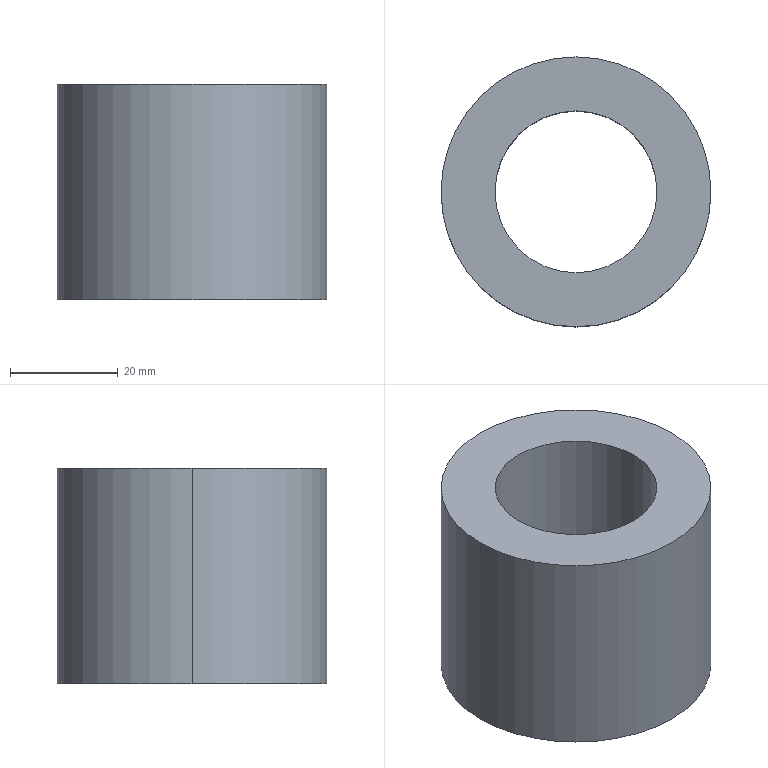Part | SolidWorks | features Extrusion 1 | 1 solid | 6 faces | box 50 x 50 x 40 mm | volume 50265 mm3 | cylinder 4 | plane 2 | commonest cylinder face diameters 30 x2 50 x2
STEP:
#1=CARTESIAN_POINT('',(-15.,0.,40.));
#2=VERTEX_POINT('',#1);
#3=CARTESIAN_POINT('',(15.,0.,40.));
#4=VERTEX_POINT('',#3);
#5=CARTESIAN_POINT('',(0.,0.,40.));
#6=DIRECTION('',(0.,0.,1.));
#7=DIRECTION('',(1.,0.,0.));
#8=AXIS2_PLACEMENT_3D('',#5,#6,#7);
#9=CIRCLE('',#8,15.);
#10=EDGE_CURVE('',#2,#4,#9,.T.);
#11=ORIENTED_EDGE('',*,*,#10,.T.);
#12=CARTESIAN_POINT('',(15.,0.,0.));
#13=VERTEX_POINT('',#12);
#14=CARTESIAN_POINT('',(15.,0.,40.));
#15=DIRECTION('',(0.,0.,-1.));
#16=VECTOR('',#15,1000.);
#17=LINE('',#14,#16);
#18=EDGE_CURVE('',#4,#13,#17,.T.);
#19=ORIENTED_EDGE('',*,*,#18,.T.);
#20=CARTESIAN_POINT('',(-15.,0.,0.));
#21=VERTEX_POINT('',#20);
#22=CARTESIAN_POINT('',(0.,0.,0.));
#23=DIRECTION('',(0.,0.,1.));
#24=DIRECTION('',(1.,0.,0.));
#25=AXIS2_PLACEMENT_3D('',#22,#23,#24);
#26=CIRCLE('',#25,15.);
#27=EDGE_CURVE('',#21,#13,#26,.T.);
#28=ORIENTED_EDGE('',*,*,#27,.F.);
#29=CARTESIAN_POINT('',(-15.,0.,40.));
#30=DIRECTION('',(0.,0.,-1.));
#31=VECTOR('',#30,1000.);
#32=LINE('',#29,#31);
#33=EDGE_CURVE('',#2,#21,#32,.T.);
#34=ORIENTED_EDGE('',*,*,#33,.F.);
#35=EDGE_LOOP('',(#11,#19,#28,#34));
#36=FACE_OUTER_BOUND('',#35,.T.);
#37=CARTESIAN_POINT('',(0.,0.,40.));
#38=DIRECTION('',(0.,0.,-1.));
#39=DIRECTION('',(-1.,0.,0.));
#40=AXIS2_PLACEMENT_3D('',#37,#38,#39);
#41=CYLINDRICAL_SURFACE('',#40,15.);
#42=ADVANCED_FACE('',(#36),#41,.F.);
#43=CARTESIAN_POINT('',(25.,0.,40.));
#44=VERTEX_POINT('',#43);
#45=CARTESIAN_POINT('',(-25.,0.,40.));
#46=VERTEX_POINT('',#45);
#47=CARTESIAN_POINT('',(0.,0.,40.));
#48=DIRECTION('',(0.,0.,1.));
#49=DIRECTION('',(1.,0.,0.));
#50=AXIS2_PLACEMENT_3D('',#47,#48,#49);
#51=CIRCLE('',#50,25.);
#52=EDGE_CURVE('',#44,#46,#51,.T.);
#53=ORIENTED_EDGE('',*,*,#52,.F.);
#54=CARTESIAN_POINT('',(25.,0.,0.));
#55=VERTEX_POINT('',#54);
#56=CARTESIAN_POINT('',(25.,0.,40.));
#57=DIRECTION('',(0.,0.,-1.));
#58=VECTOR('',#57,1000.);
#59=LINE('',#56,#58);
#60=EDGE_CURVE('',#44,#55,#59,.T.);
#61=ORIENTED_EDGE('',*,*,#60,.T.);
#62=CARTESIAN_POINT('',(-25.,0.,0.));
#63=VERTEX_POINT('',#62);
#64=CARTESIAN_POINT('',(0.,0.,0.));
#65=DIRECTION('',(0.,0.,1.));
#66=DIRECTION('',(1.,0.,0.));
#67=AXIS2_PLACEMENT_3D('',#64,#65,#66);
#68=CIRCLE('',#67,25.);
#69=EDGE_CURVE('',#55,#63,#68,.T.);
#70=ORIENTED_EDGE('',*,*,#69,.T.);
#71=CARTESIAN_POINT('',(-25.,0.,40.));
#72=DIRECTION('',(0.,0.,-1.));
#73=VECTOR('',#72,1000.);
#74=LINE('',#71,#73);
#75=EDGE_CURVE('',#46,#63,#74,.T.);
#76=ORIENTED_EDGE('',*,*,#75,.F.);
#77=EDGE_LOOP('',(#53,#61,#70,#76));
#78=FACE_OUTER_BOUND('',#77,.T.);
#79=CARTESIAN_POINT('',(0.,0.,40.));
#80=DIRECTION('',(0.,0.,-1.));
#81=DIRECTION('',(-1.,0.,0.));
#82=AXIS2_PLACEMENT_3D('',#79,#80,#81);
#83=CYLINDRICAL_SURFACE('',#82,25.);
#84=ADVANCED_FACE('',(#78),#83,.T.);
#85=CARTESIAN_POINT('',(0.,0.,40.));
#86=DIRECTION('',(0.,0.,1.));
#87=DIRECTION('',(1.,0.,0.));
#88=AXIS2_PLACEMENT_3D('',#85,#86,#87);
#89=CIRCLE('',#88,25.);
#90=EDGE_CURVE('',#46,#44,#89,.T.);
#91=ORIENTED_EDGE('',*,*,#90,.T.);
#92=ORIENTED_EDGE('',*,*,#52,.T.);
#93=EDGE_LOOP('',(#91,#92));
#94=FACE_OUTER_BOUND('',#93,.T.);
#95=ORIENTED_EDGE('',*,*,#10,.F.);
#96=CARTESIAN_POINT('',(0.,0.,40.));
#97=DIRECTION('',(0.,0.,1.));
#98=DIRECTION('',(1.,0.,0.));
#99=AXIS2_PLACEMENT_3D('',#96,#97,#98);
#100=CIRCLE('',#99,15.);
#101=EDGE_CURVE('',#4,#2,#100,.T.);
#102=ORIENTED_EDGE('',*,*,#101,.F.);
#103=EDGE_LOOP('',(#95,#102));
#104=FACE_BOUND('',#103,.T.);
#105=CARTESIAN_POINT('',(0.,0.,40.));
#106=DIRECTION('',(0.,0.,1.));
#107=DIRECTION('',(1.,0.,0.));
#108=AXIS2_PLACEMENT_3D('',#105,#106,#107);
#109=PLANE('',#108);
#110=ADVANCED_FACE('',(#94,#104),#109,.T.);
#111=CARTESIAN_POINT('',(0.,0.,0.));
#112=DIRECTION('',(0.,0.,1.));
#113=DIRECTION('',(1.,0.,0.));
#114=AXIS2_PLACEMENT_3D('',#111,#112,#113);
#115=CIRCLE('',#114,25.);
#116=EDGE_CURVE('',#63,#55,#115,.T.);
#117=ORIENTED_EDGE('',*,*,#116,.F.);
#118=ORIENTED_EDGE('',*,*,#69,.F.);
#119=EDGE_LOOP('',(#117,#118));
#120=FACE_OUTER_BOUND('',#119,.T.);
#121=ORIENTED_EDGE('',*,*,#27,.T.);
#122=CARTESIAN_POINT('',(0.,0.,0.));
#123=DIRECTION('',(0.,0.,1.));
#124=DIRECTION('',(1.,0.,0.));
#125=AXIS2_PLACEMENT_3D('',#122,#123,#124);
#126=CIRCLE('',#125,15.);
#127=EDGE_CURVE('',#13,#21,#126,.T.);
#128=ORIENTED_EDGE('',*,*,#127,.T.);
#129=EDGE_LOOP('',(#121,#128));
#130=FACE_BOUND('',#129,.T.);
#131=CARTESIAN_POINT('',(0.,0.,0.));
#132=DIRECTION('',(0.,0.,1.));
#133=DIRECTION('',(1.,0.,0.));
#134=AXIS2_PLACEMENT_3D('',#131,#132,#133);
#135=PLANE('',#134);
#136=ADVANCED_FACE('',(#120,#130),#135,.F.);
#137=ORIENTED_EDGE('',*,*,#60,.F.);
#138=ORIENTED_EDGE('',*,*,#90,.F.);
#139=ORIENTED_EDGE('',*,*,#75,.T.);
#140=ORIENTED_EDGE('',*,*,#116,.T.);
#141=EDGE_LOOP('',(#137,#138,#139,#140));
#142=FACE_OUTER_BOUND('',#141,.T.);
#143=CARTESIAN_POINT('',(0.,0.,40.));
#144=DIRECTION('',(0.,0.,-1.));
#145=DIRECTION('',(-1.,0.,0.));
#146=AXIS2_PLACEMENT_3D('',#143,#144,#145);
#147=CYLINDRICAL_SURFACE('',#146,25.);
#148=ADVANCED_FACE('',(#142),#147,.T.);
#149=ORIENTED_EDGE('',*,*,#18,.F.);
#150=ORIENTED_EDGE('',*,*,#101,.T.);
#151=ORIENTED_EDGE('',*,*,#33,.T.);
#152=ORIENTED_EDGE('',*,*,#127,.F.);
#153=EDGE_LOOP('',(#149,#150,#151,#152));
#154=FACE_OUTER_BOUND('',#153,.T.);
#155=CARTESIAN_POINT('',(0.,0.,40.));
#156=DIRECTION('',(0.,0.,-1.));
#157=DIRECTION('',(-1.,0.,0.));
#158=AXIS2_PLACEMENT_3D('',#155,#156,#157);
#159=CYLINDRICAL_SURFACE('',#158,15.);
#160=ADVANCED_FACE('',(#154),#159,.F.);
#161=CLOSED_SHELL('',(#42,#84,#110,#136,#148,#160));
#162=MANIFOLD_SOLID_BREP('',#161);
#163=CARTESIAN_POINT('',(0.,0.,0.));
#164=DIRECTION('',(0.,0.,1.));
#165=DIRECTION('',(1.,0.,0.));
#166=AXIS2_PLACEMENT_3D('',#163,#164,#165);
#167=(LENGTH_UNIT()NAMED_UNIT(*)SI_UNIT(.MILLI.,.METRE.));
#168=UNCERTAINTY_MEASURE_WITH_UNIT(LENGTH_MEASURE(0.00001),#167,'','');
#169=(NAMED_UNIT(*)PLANE_ANGLE_UNIT()SI_UNIT($,.RADIAN.));
#170=(NAMED_UNIT(*)SI_UNIT($,.STERADIAN.)SOLID_ANGLE_UNIT());
#171=(GEOMETRIC_REPRESENTATION_CONTEXT(3)GLOBAL_UNCERTAINTY_ASSIGNED_CONTEXT((#168))GLOBAL_UNIT_ASSIGNED_CONTEXT((#167,#169,#170))REPRESENTATION_CONTEXT('',''));
#172=ADVANCED_BREP_SHAPE_REPRESENTATION('',(#162,#166),#171);